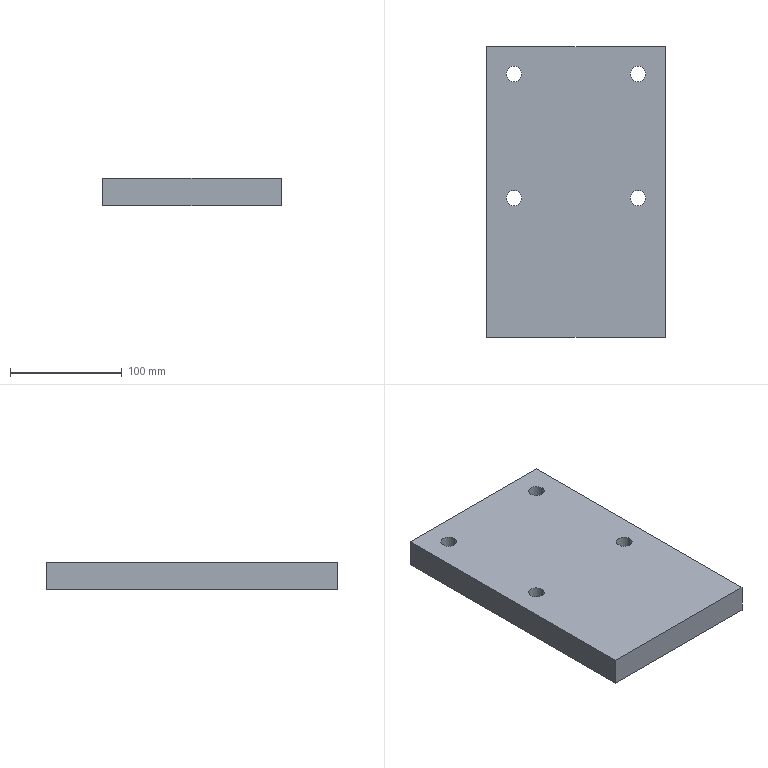Part | SolidWorks | features Extrusion 1, HoleWzd 1 | 1 solid | 14 faces | box 160 x 260 x 25 mm | volume 1024606 mm3 | cylinder 8 | plane 6 | commonest cylinder face diameters 14 x8
STEP:
#1=CARTESIAN_POINT('',(-62.5,105.5,0.));
#2=VERTEX_POINT('',#1);
#3=CARTESIAN_POINT('',(-48.5,105.5,0.));
#4=VERTEX_POINT('',#3);
#5=CARTESIAN_POINT('',(-55.5,105.5,0.));
#6=DIRECTION('',(0.,0.,1.));
#7=DIRECTION('',(1.,0.,0.));
#8=AXIS2_PLACEMENT_3D('',#5,#6,#7);
#9=CIRCLE('',#8,7.);
#10=EDGE_CURVE('',#2,#4,#9,.T.);
#11=ORIENTED_EDGE('',*,*,#10,.F.);
#12=CARTESIAN_POINT('',(-62.5,105.5,25.));
#13=VERTEX_POINT('',#12);
#14=CARTESIAN_POINT('',(-62.5,105.5,25.));
#15=DIRECTION('',(0.,0.,1.));
#16=VECTOR('',#15,1000.);
#17=LINE('',#14,#16);
#18=EDGE_CURVE('',#2,#13,#17,.T.);
#19=ORIENTED_EDGE('',*,*,#18,.T.);
#20=CARTESIAN_POINT('',(-48.5,105.5,25.));
#21=VERTEX_POINT('',#20);
#22=CARTESIAN_POINT('',(-55.5,105.5,25.));
#23=DIRECTION('',(0.,0.,1.));
#24=DIRECTION('',(1.,0.,0.));
#25=AXIS2_PLACEMENT_3D('',#22,#23,#24);
#26=CIRCLE('',#25,7.);
#27=EDGE_CURVE('',#13,#21,#26,.T.);
#28=ORIENTED_EDGE('',*,*,#27,.T.);
#29=CARTESIAN_POINT('',(-48.5,105.5,25.));
#30=DIRECTION('',(0.,0.,1.));
#31=VECTOR('',#30,1000.);
#32=LINE('',#29,#31);
#33=EDGE_CURVE('',#4,#21,#32,.T.);
#34=ORIENTED_EDGE('',*,*,#33,.F.);
#35=EDGE_LOOP('',(#11,#19,#28,#34));
#36=FACE_OUTER_BOUND('',#35,.T.);
#37=CARTESIAN_POINT('',(-55.5,105.5,25.));
#38=DIRECTION('',(0.,0.,1.));
#39=DIRECTION('',(1.,0.,0.));
#40=AXIS2_PLACEMENT_3D('',#37,#38,#39);
#41=CYLINDRICAL_SURFACE('',#40,7.);
#42=ADVANCED_FACE('',(#36),#41,.F.);
#43=CARTESIAN_POINT('',(-62.5,-5.5,0.));
#44=VERTEX_POINT('',#43);
#45=CARTESIAN_POINT('',(-48.5,-5.5,0.));
#46=VERTEX_POINT('',#45);
#47=CARTESIAN_POINT('',(-55.5,-5.5,0.));
#48=DIRECTION('',(0.,0.,1.));
#49=DIRECTION('',(1.,0.,0.));
#50=AXIS2_PLACEMENT_3D('',#47,#48,#49);
#51=CIRCLE('',#50,7.);
#52=EDGE_CURVE('',#44,#46,#51,.T.);
#53=ORIENTED_EDGE('',*,*,#52,.F.);
#54=CARTESIAN_POINT('',(-62.5,-5.5,25.));
#55=VERTEX_POINT('',#54);
#56=CARTESIAN_POINT('',(-62.5,-5.5,25.));
#57=DIRECTION('',(0.,0.,1.));
#58=VECTOR('',#57,1000.);
#59=LINE('',#56,#58);
#60=EDGE_CURVE('',#44,#55,#59,.T.);
#61=ORIENTED_EDGE('',*,*,#60,.T.);
#62=CARTESIAN_POINT('',(-48.5,-5.5,25.));
#63=VERTEX_POINT('',#62);
#64=CARTESIAN_POINT('',(-55.5,-5.5,25.));
#65=DIRECTION('',(0.,0.,1.));
#66=DIRECTION('',(1.,0.,0.));
#67=AXIS2_PLACEMENT_3D('',#64,#65,#66);
#68=CIRCLE('',#67,7.);
#69=EDGE_CURVE('',#55,#63,#68,.T.);
#70=ORIENTED_EDGE('',*,*,#69,.T.);
#71=CARTESIAN_POINT('',(-48.5,-5.5,25.));
#72=DIRECTION('',(0.,0.,1.));
#73=VECTOR('',#72,1000.);
#74=LINE('',#71,#73);
#75=EDGE_CURVE('',#46,#63,#74,.T.);
#76=ORIENTED_EDGE('',*,*,#75,.F.);
#77=EDGE_LOOP('',(#53,#61,#70,#76));
#78=FACE_OUTER_BOUND('',#77,.T.);
#79=CARTESIAN_POINT('',(-55.5,-5.5,25.));
#80=DIRECTION('',(0.,0.,1.));
#81=DIRECTION('',(1.,0.,0.));
#82=AXIS2_PLACEMENT_3D('',#79,#80,#81);
#83=CYLINDRICAL_SURFACE('',#82,7.);
#84=ADVANCED_FACE('',(#78),#83,.F.);
#85=CARTESIAN_POINT('',(48.5,-5.5,0.));
#86=VERTEX_POINT('',#85);
#87=CARTESIAN_POINT('',(62.5,-5.5,0.));
#88=VERTEX_POINT('',#87);
#89=CARTESIAN_POINT('',(55.5,-5.5,0.));
#90=DIRECTION('',(0.,0.,1.));
#91=DIRECTION('',(1.,0.,0.));
#92=AXIS2_PLACEMENT_3D('',#89,#90,#91);
#93=CIRCLE('',#92,7.);
#94=EDGE_CURVE('',#86,#88,#93,.T.);
#95=ORIENTED_EDGE('',*,*,#94,.F.);
#96=CARTESIAN_POINT('',(48.5,-5.5,25.));
#97=VERTEX_POINT('',#96);
#98=CARTESIAN_POINT('',(48.5,-5.5,25.));
#99=DIRECTION('',(0.,0.,1.));
#100=VECTOR('',#99,1000.);
#101=LINE('',#98,#100);
#102=EDGE_CURVE('',#86,#97,#101,.T.);
#103=ORIENTED_EDGE('',*,*,#102,.T.);
#104=CARTESIAN_POINT('',(62.5,-5.5,25.));
#105=VERTEX_POINT('',#104);
#106=CARTESIAN_POINT('',(55.5,-5.5,25.));
#107=DIRECTION('',(0.,0.,1.));
#108=DIRECTION('',(1.,0.,0.));
#109=AXIS2_PLACEMENT_3D('',#106,#107,#108);
#110=CIRCLE('',#109,7.);
#111=EDGE_CURVE('',#97,#105,#110,.T.);
#112=ORIENTED_EDGE('',*,*,#111,.T.);
#113=CARTESIAN_POINT('',(62.5,-5.5,25.));
#114=DIRECTION('',(0.,0.,1.));
#115=VECTOR('',#114,1000.);
#116=LINE('',#113,#115);
#117=EDGE_CURVE('',#88,#105,#116,.T.);
#118=ORIENTED_EDGE('',*,*,#117,.F.);
#119=EDGE_LOOP('',(#95,#103,#112,#118));
#120=FACE_OUTER_BOUND('',#119,.T.);
#121=CARTESIAN_POINT('',(55.5,-5.5,25.));
#122=DIRECTION('',(0.,0.,1.));
#123=DIRECTION('',(1.,0.,0.));
#124=AXIS2_PLACEMENT_3D('',#121,#122,#123);
#125=CYLINDRICAL_SURFACE('',#124,7.);
#126=ADVANCED_FACE('',(#120),#125,.F.);
#127=CARTESIAN_POINT('',(48.5,105.5,0.));
#128=VERTEX_POINT('',#127);
#129=CARTESIAN_POINT('',(62.5,105.5,0.));
#130=VERTEX_POINT('',#129);
#131=CARTESIAN_POINT('',(55.5,105.5,0.));
#132=DIRECTION('',(0.,0.,1.));
#133=DIRECTION('',(1.,0.,0.));
#134=AXIS2_PLACEMENT_3D('',#131,#132,#133);
#135=CIRCLE('',#134,7.);
#136=EDGE_CURVE('',#128,#130,#135,.T.);
#137=ORIENTED_EDGE('',*,*,#136,.F.);
#138=CARTESIAN_POINT('',(48.5,105.5,25.));
#139=VERTEX_POINT('',#138);
#140=CARTESIAN_POINT('',(48.5,105.5,25.));
#141=DIRECTION('',(0.,0.,1.));
#142=VECTOR('',#141,1000.);
#143=LINE('',#140,#142);
#144=EDGE_CURVE('',#128,#139,#143,.T.);
#145=ORIENTED_EDGE('',*,*,#144,.T.);
#146=CARTESIAN_POINT('',(62.5,105.5,25.));
#147=VERTEX_POINT('',#146);
#148=CARTESIAN_POINT('',(55.5,105.5,25.));
#149=DIRECTION('',(0.,0.,1.));
#150=DIRECTION('',(1.,0.,0.));
#151=AXIS2_PLACEMENT_3D('',#148,#149,#150);
#152=CIRCLE('',#151,7.);
#153=EDGE_CURVE('',#139,#147,#152,.T.);
#154=ORIENTED_EDGE('',*,*,#153,.T.);
#155=CARTESIAN_POINT('',(62.5,105.5,25.));
#156=DIRECTION('',(0.,0.,1.));
#157=VECTOR('',#156,1000.);
#158=LINE('',#155,#157);
#159=EDGE_CURVE('',#130,#147,#158,.T.);
#160=ORIENTED_EDGE('',*,*,#159,.F.);
#161=EDGE_LOOP('',(#137,#145,#154,#160));
#162=FACE_OUTER_BOUND('',#161,.T.);
#163=CARTESIAN_POINT('',(55.5,105.5,25.));
#164=DIRECTION('',(0.,0.,1.));
#165=DIRECTION('',(1.,0.,0.));
#166=AXIS2_PLACEMENT_3D('',#163,#164,#165);
#167=CYLINDRICAL_SURFACE('',#166,7.);
#168=ADVANCED_FACE('',(#162),#167,.F.);
#169=CARTESIAN_POINT('',(-80.,130.,0.));
#170=VERTEX_POINT('',#169);
#171=CARTESIAN_POINT('',(-80.,-130.,0.));
#172=VERTEX_POINT('',#171);
#173=CARTESIAN_POINT('',(-80.,-130.,0.));
#174=DIRECTION('',(0.,-1.,0.));
#175=VECTOR('',#174,1000.);
#176=LINE('',#173,#175);
#177=EDGE_CURVE('',#170,#172,#176,.T.);
#178=ORIENTED_EDGE('',*,*,#177,.T.);
#179=CARTESIAN_POINT('',(-80.,-130.,25.));
#180=VERTEX_POINT('',#179);
#181=CARTESIAN_POINT('',(-80.,-130.,25.));
#182=DIRECTION('',(0.,0.,-1.));
#183=VECTOR('',#182,1000.);
#184=LINE('',#181,#183);
#185=EDGE_CURVE('',#180,#172,#184,.T.);
#186=ORIENTED_EDGE('',*,*,#185,.F.);
#187=CARTESIAN_POINT('',(-80.,130.,25.));
#188=VERTEX_POINT('',#187);
#189=CARTESIAN_POINT('',(-80.,-130.,25.));
#190=DIRECTION('',(0.,-1.,0.));
#191=VECTOR('',#190,1000.);
#192=LINE('',#189,#191);
#193=EDGE_CURVE('',#188,#180,#192,.T.);
#194=ORIENTED_EDGE('',*,*,#193,.F.);
#195=CARTESIAN_POINT('',(-80.,130.,25.));
#196=DIRECTION('',(0.,0.,-1.));
#197=VECTOR('',#196,1000.);
#198=LINE('',#195,#197);
#199=EDGE_CURVE('',#188,#170,#198,.T.);
#200=ORIENTED_EDGE('',*,*,#199,.T.);
#201=EDGE_LOOP('',(#178,#186,#194,#200));
#202=FACE_OUTER_BOUND('',#201,.T.);
#203=CARTESIAN_POINT('',(-80.,-130.,25.));
#204=DIRECTION('',(1.,0.,0.));
#205=DIRECTION('',(0.,0.,-1.));
#206=AXIS2_PLACEMENT_3D('',#203,#204,#205);
#207=PLANE('',#206);
#208=ADVANCED_FACE('',(#202),#207,.F.);
#209=CARTESIAN_POINT('',(80.,-130.,0.));
#210=VERTEX_POINT('',#209);
#211=CARTESIAN_POINT('',(80.,-130.,0.));
#212=DIRECTION('',(1.,0.,0.));
#213=VECTOR('',#212,1000.);
#214=LINE('',#211,#213);
#215=EDGE_CURVE('',#172,#210,#214,.T.);
#216=ORIENTED_EDGE('',*,*,#215,.T.);
#217=CARTESIAN_POINT('',(80.,-130.,25.));
#218=VERTEX_POINT('',#217);
#219=CARTESIAN_POINT('',(80.,-130.,25.));
#220=DIRECTION('',(0.,0.,-1.));
#221=VECTOR('',#220,1000.);
#222=LINE('',#219,#221);
#223=EDGE_CURVE('',#218,#210,#222,.T.);
#224=ORIENTED_EDGE('',*,*,#223,.F.);
#225=CARTESIAN_POINT('',(80.,-130.,25.));
#226=DIRECTION('',(1.,0.,0.));
#227=VECTOR('',#226,1000.);
#228=LINE('',#225,#227);
#229=EDGE_CURVE('',#180,#218,#228,.T.);
#230=ORIENTED_EDGE('',*,*,#229,.F.);
#231=ORIENTED_EDGE('',*,*,#185,.T.);
#232=EDGE_LOOP('',(#216,#224,#230,#231));
#233=FACE_OUTER_BOUND('',#232,.T.);
#234=CARTESIAN_POINT('',(80.,-130.,25.));
#235=DIRECTION('',(0.,1.,0.));
#236=DIRECTION('',(-1.,0.,0.));
#237=AXIS2_PLACEMENT_3D('',#234,#235,#236);
#238=PLANE('',#237);
#239=ADVANCED_FACE('',(#233),#238,.F.);
#240=CARTESIAN_POINT('',(80.,130.,0.));
#241=VERTEX_POINT('',#240);
#242=CARTESIAN_POINT('',(80.,-130.,0.));
#243=DIRECTION('',(0.,1.,0.));
#244=VECTOR('',#243,1000.);
#245=LINE('',#242,#244);
#246=EDGE_CURVE('',#210,#241,#245,.T.);
#247=ORIENTED_EDGE('',*,*,#246,.T.);
#248=CARTESIAN_POINT('',(80.,130.,25.));
#249=VERTEX_POINT('',#248);
#250=CARTESIAN_POINT('',(80.,130.,25.));
#251=DIRECTION('',(0.,0.,-1.));
#252=VECTOR('',#251,1000.);
#253=LINE('',#250,#252);
#254=EDGE_CURVE('',#249,#241,#253,.T.);
#255=ORIENTED_EDGE('',*,*,#254,.F.);
#256=CARTESIAN_POINT('',(80.,-130.,25.));
#257=DIRECTION('',(0.,1.,0.));
#258=VECTOR('',#257,1000.);
#259=LINE('',#256,#258);
#260=EDGE_CURVE('',#218,#249,#259,.T.);
#261=ORIENTED_EDGE('',*,*,#260,.F.);
#262=ORIENTED_EDGE('',*,*,#223,.T.);
#263=EDGE_LOOP('',(#247,#255,#261,#262));
#264=FACE_OUTER_BOUND('',#263,.T.);
#265=CARTESIAN_POINT('',(80.,-130.,25.));
#266=DIRECTION('',(-1.,0.,0.));
#267=DIRECTION('',(0.,-1.,0.));
#268=AXIS2_PLACEMENT_3D('',#265,#266,#267);
#269=PLANE('',#268);
#270=ADVANCED_FACE('',(#264),#269,.F.);
#271=CARTESIAN_POINT('',(80.,130.,0.));
#272=DIRECTION('',(-1.,0.,0.));
#273=VECTOR('',#272,1000.);
#274=LINE('',#271,#273);
#275=EDGE_CURVE('',#241,#170,#274,.T.);
#276=ORIENTED_EDGE('',*,*,#275,.T.);
#277=ORIENTED_EDGE('',*,*,#199,.F.);
#278=CARTESIAN_POINT('',(80.,130.,25.));
#279=DIRECTION('',(-1.,0.,0.));
#280=VECTOR('',#279,1000.);
#281=LINE('',#278,#280);
#282=EDGE_CURVE('',#249,#188,#281,.T.);
#283=ORIENTED_EDGE('',*,*,#282,.F.);
#284=ORIENTED_EDGE('',*,*,#254,.T.);
#285=EDGE_LOOP('',(#276,#277,#283,#284));
#286=FACE_OUTER_BOUND('',#285,.T.);
#287=CARTESIAN_POINT('',(80.,130.,25.));
#288=DIRECTION('',(0.,-1.,0.));
#289=DIRECTION('',(0.,0.,-1.));
#290=AXIS2_PLACEMENT_3D('',#287,#288,#289);
#291=PLANE('',#290);
#292=ADVANCED_FACE('',(#286),#291,.F.);
#293=CARTESIAN_POINT('',(-55.5,105.5,25.));
#294=DIRECTION('',(0.,0.,1.));
#295=DIRECTION('',(1.,0.,0.));
#296=AXIS2_PLACEMENT_3D('',#293,#294,#295);
#297=CIRCLE('',#296,7.);
#298=EDGE_CURVE('',#21,#13,#297,.T.);
#299=ORIENTED_EDGE('',*,*,#298,.F.);
#300=ORIENTED_EDGE('',*,*,#27,.F.);
#301=EDGE_LOOP('',(#299,#300));
#302=FACE_BOUND('',#301,.T.);
#303=CARTESIAN_POINT('',(-55.5,-5.5,25.));
#304=DIRECTION('',(0.,0.,1.));
#305=DIRECTION('',(1.,0.,0.));
#306=AXIS2_PLACEMENT_3D('',#303,#304,#305);
#307=CIRCLE('',#306,7.);
#308=EDGE_CURVE('',#63,#55,#307,.T.);
#309=ORIENTED_EDGE('',*,*,#308,.F.);
#310=ORIENTED_EDGE('',*,*,#69,.F.);
#311=EDGE_LOOP('',(#309,#310));
#312=FACE_BOUND('',#311,.T.);
#313=CARTESIAN_POINT('',(55.5,-5.5,25.));
#314=DIRECTION('',(0.,0.,1.));
#315=DIRECTION('',(1.,0.,0.));
#316=AXIS2_PLACEMENT_3D('',#313,#314,#315);
#317=CIRCLE('',#316,7.);
#318=EDGE_CURVE('',#105,#97,#317,.T.);
#319=ORIENTED_EDGE('',*,*,#318,.F.);
#320=ORIENTED_EDGE('',*,*,#111,.F.);
#321=EDGE_LOOP('',(#319,#320));
#322=FACE_BOUND('',#321,.T.);
#323=CARTESIAN_POINT('',(55.5,105.5,25.));
#324=DIRECTION('',(0.,0.,1.));
#325=DIRECTION('',(1.,0.,0.));
#326=AXIS2_PLACEMENT_3D('',#323,#324,#325);
#327=CIRCLE('',#326,7.);
#328=EDGE_CURVE('',#147,#139,#327,.T.);
#329=ORIENTED_EDGE('',*,*,#328,.F.);
#330=ORIENTED_EDGE('',*,*,#153,.F.);
#331=EDGE_LOOP('',(#329,#330));
#332=FACE_BOUND('',#331,.T.);
#333=ORIENTED_EDGE('',*,*,#193,.T.);
#334=ORIENTED_EDGE('',*,*,#229,.T.);
#335=ORIENTED_EDGE('',*,*,#260,.T.);
#336=ORIENTED_EDGE('',*,*,#282,.T.);
#337=EDGE_LOOP('',(#333,#334,#335,#336));
#338=FACE_OUTER_BOUND('',#337,.T.);
#339=CARTESIAN_POINT('',(0.,0.,25.));
#340=DIRECTION('',(0.,0.,1.));
#341=DIRECTION('',(1.,0.,0.));
#342=AXIS2_PLACEMENT_3D('',#339,#340,#341);
#343=PLANE('',#342);
#344=ADVANCED_FACE('',(#302,#312,#322,#332,#338),#343,.T.);
#345=CARTESIAN_POINT('',(-55.5,105.5,0.));
#346=DIRECTION('',(0.,0.,1.));
#347=DIRECTION('',(1.,0.,0.));
#348=AXIS2_PLACEMENT_3D('',#345,#346,#347);
#349=CIRCLE('',#348,7.);
#350=EDGE_CURVE('',#4,#2,#349,.T.);
#351=ORIENTED_EDGE('',*,*,#350,.T.);
#352=ORIENTED_EDGE('',*,*,#10,.T.);
#353=EDGE_LOOP('',(#351,#352));
#354=FACE_BOUND('',#353,.T.);
#355=CARTESIAN_POINT('',(-55.5,-5.5,0.));
#356=DIRECTION('',(0.,0.,1.));
#357=DIRECTION('',(1.,0.,0.));
#358=AXIS2_PLACEMENT_3D('',#355,#356,#357);
#359=CIRCLE('',#358,7.);
#360=EDGE_CURVE('',#46,#44,#359,.T.);
#361=ORIENTED_EDGE('',*,*,#360,.T.);
#362=ORIENTED_EDGE('',*,*,#52,.T.);
#363=EDGE_LOOP('',(#361,#362));
#364=FACE_BOUND('',#363,.T.);
#365=CARTESIAN_POINT('',(55.5,-5.5,0.));
#366=DIRECTION('',(0.,0.,1.));
#367=DIRECTION('',(1.,0.,0.));
#368=AXIS2_PLACEMENT_3D('',#365,#366,#367);
#369=CIRCLE('',#368,7.);
#370=EDGE_CURVE('',#88,#86,#369,.T.);
#371=ORIENTED_EDGE('',*,*,#370,.T.);
#372=ORIENTED_EDGE('',*,*,#94,.T.);
#373=EDGE_LOOP('',(#371,#372));
#374=FACE_BOUND('',#373,.T.);
#375=CARTESIAN_POINT('',(55.5,105.5,0.));
#376=DIRECTION('',(0.,0.,1.));
#377=DIRECTION('',(1.,0.,0.));
#378=AXIS2_PLACEMENT_3D('',#375,#376,#377);
#379=CIRCLE('',#378,7.);
#380=EDGE_CURVE('',#130,#128,#379,.T.);
#381=ORIENTED_EDGE('',*,*,#380,.T.);
#382=ORIENTED_EDGE('',*,*,#136,.T.);
#383=EDGE_LOOP('',(#381,#382));
#384=FACE_BOUND('',#383,.T.);
#385=ORIENTED_EDGE('',*,*,#177,.F.);
#386=ORIENTED_EDGE('',*,*,#275,.F.);
#387=ORIENTED_EDGE('',*,*,#246,.F.);
#388=ORIENTED_EDGE('',*,*,#215,.F.);
#389=EDGE_LOOP('',(#385,#386,#387,#388));
#390=FACE_OUTER_BOUND('',#389,.T.);
#391=CARTESIAN_POINT('',(0.,0.,0.));
#392=DIRECTION('',(0.,0.,1.));
#393=DIRECTION('',(1.,0.,0.));
#394=AXIS2_PLACEMENT_3D('',#391,#392,#393);
#395=PLANE('',#394);
#396=ADVANCED_FACE('',(#354,#364,#374,#384,#390),#395,.F.);
#397=ORIENTED_EDGE('',*,*,#144,.F.);
#398=ORIENTED_EDGE('',*,*,#380,.F.);
#399=ORIENTED_EDGE('',*,*,#159,.T.);
#400=ORIENTED_EDGE('',*,*,#328,.T.);
#401=EDGE_LOOP('',(#397,#398,#399,#400));
#402=FACE_OUTER_BOUND('',#401,.T.);
#403=CARTESIAN_POINT('',(55.5,105.5,25.));
#404=DIRECTION('',(0.,0.,1.));
#405=DIRECTION('',(1.,0.,0.));
#406=AXIS2_PLACEMENT_3D('',#403,#404,#405);
#407=CYLINDRICAL_SURFACE('',#406,7.);
#408=ADVANCED_FACE('',(#402),#407,.F.);
#409=ORIENTED_EDGE('',*,*,#102,.F.);
#410=ORIENTED_EDGE('',*,*,#370,.F.);
#411=ORIENTED_EDGE('',*,*,#117,.T.);
#412=ORIENTED_EDGE('',*,*,#318,.T.);
#413=EDGE_LOOP('',(#409,#410,#411,#412));
#414=FACE_OUTER_BOUND('',#413,.T.);
#415=CARTESIAN_POINT('',(55.5,-5.5,25.));
#416=DIRECTION('',(0.,0.,1.));
#417=DIRECTION('',(1.,0.,0.));
#418=AXIS2_PLACEMENT_3D('',#415,#416,#417);
#419=CYLINDRICAL_SURFACE('',#418,7.);
#420=ADVANCED_FACE('',(#414),#419,.F.);
#421=ORIENTED_EDGE('',*,*,#60,.F.);
#422=ORIENTED_EDGE('',*,*,#360,.F.);
#423=ORIENTED_EDGE('',*,*,#75,.T.);
#424=ORIENTED_EDGE('',*,*,#308,.T.);
#425=EDGE_LOOP('',(#421,#422,#423,#424));
#426=FACE_OUTER_BOUND('',#425,.T.);
#427=CARTESIAN_POINT('',(-55.5,-5.5,25.));
#428=DIRECTION('',(0.,0.,1.));
#429=DIRECTION('',(1.,0.,0.));
#430=AXIS2_PLACEMENT_3D('',#427,#428,#429);
#431=CYLINDRICAL_SURFACE('',#430,7.);
#432=ADVANCED_FACE('',(#426),#431,.F.);
#433=ORIENTED_EDGE('',*,*,#18,.F.);
#434=ORIENTED_EDGE('',*,*,#350,.F.);
#435=ORIENTED_EDGE('',*,*,#33,.T.);
#436=ORIENTED_EDGE('',*,*,#298,.T.);
#437=EDGE_LOOP('',(#433,#434,#435,#436));
#438=FACE_OUTER_BOUND('',#437,.T.);
#439=CARTESIAN_POINT('',(-55.5,105.5,25.));
#440=DIRECTION('',(0.,0.,1.));
#441=DIRECTION('',(1.,0.,0.));
#442=AXIS2_PLACEMENT_3D('',#439,#440,#441);
#443=CYLINDRICAL_SURFACE('',#442,7.);
#444=ADVANCED_FACE('',(#438),#443,.F.);
#445=CLOSED_SHELL('',(#42,#84,#126,#168,#208,#239,#270,#292,#344,#396,#408,#420,#432,#444));
#446=MANIFOLD_SOLID_BREP('',#445);
#447=CARTESIAN_POINT('',(0.,0.,0.));
#448=DIRECTION('',(0.,0.,1.));
#449=DIRECTION('',(1.,0.,0.));
#450=AXIS2_PLACEMENT_3D('',#447,#448,#449);
#451=(LENGTH_UNIT()NAMED_UNIT(*)SI_UNIT(.MILLI.,.METRE.));
#452=UNCERTAINTY_MEASURE_WITH_UNIT(LENGTH_MEASURE(0.00001),#451,'','');
#453=(NAMED_UNIT(*)PLANE_ANGLE_UNIT()SI_UNIT($,.RADIAN.));
#454=(NAMED_UNIT(*)SI_UNIT($,.STERADIAN.)SOLID_ANGLE_UNIT());
#455=(GEOMETRIC_REPRESENTATION_CONTEXT(3)GLOBAL_UNCERTAINTY_ASSIGNED_CONTEXT((#452))GLOBAL_UNIT_ASSIGNED_CONTEXT((#451,#453,#454))REPRESENTATION_CONTEXT('',''));
#456=ADVANCED_BREP_SHAPE_REPRESENTATION('',(#446,#450),#455);